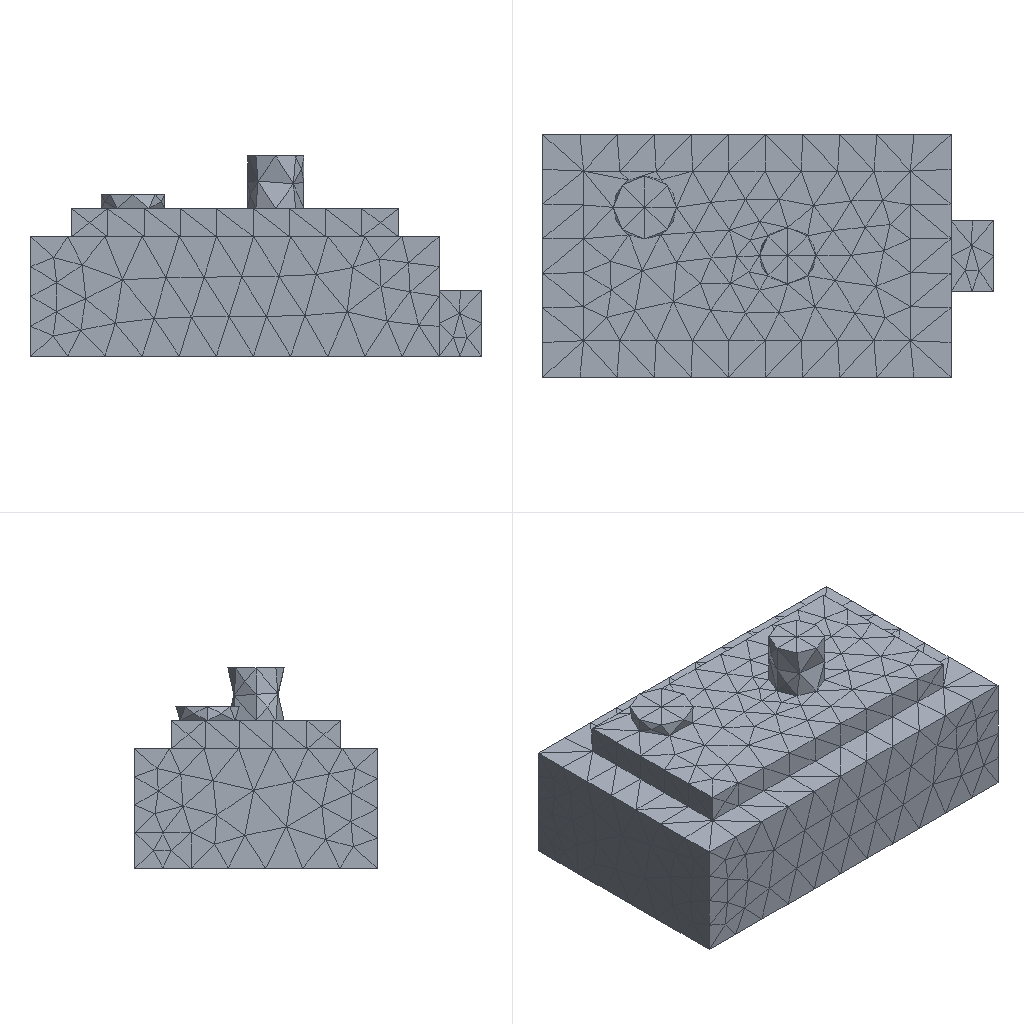Simulation study | ansys mapdl
Set-up summary:
category,name,step,type,value,unit,region
solver,ansys_mapdl
units,mm-N-s-tonne (MPa),,inferred,E=210000 density=
analysis,model,,static
mesh,nodes,,,4669
mesh,elements,,,2793
element_type,SOLID187,,,2793
material,mat 1,,E,210000
material,mat 1,,nu,0.3
load,,model,body load temp,,,all
load,,model,force,"1000 [dir=(0, 0, -1) n=93]",,node list
bc,,model,fixed,"[dofs=UX,UY,UZ n=4945]",,node list
Ansys APDL input file, long lists of numbers shortened:
/COM,ANSYS RELEASE 2026 R1           BUILD 26.1      UP20260202       09:08:28
/PREP7
/NOPR
/TITLE,2
ANTYPE, 0
*IF,_CDRDOFF,EQ,1,THEN     !if solid model was read in
_CDRDOFF=             !reset flag, numoffs already performed
*ELSE              !offset database for the following FE model
NUMOFF,NODE,     4669
NUMOFF,ELEM,     2793
NUMOFF,MAT ,        1
NUMOFF,TYPE,        1
*ENDIF
*SET,_RETURN ,  0.
*SET,_STATUS ,  0.
*SET,_UIQR   ,  93.
*SET,__FLOATPARAMETER__,  4669.
DOF,DELETE
ETBLOCK,        1,        1
(2i9,19a9)
        1      187        0        0        0        0        0        0        0        0        0        0        0        0        0        0        0        0        0        0        0
       -1
NBLOCK,6,SOLID,      4669,      4669
(3i9,6e21.13e3)
        1        0        0-4.2125000000000E+001 3.4500000000000E+001 1.0000000000000E+001
! (4668 more lines like these left out)
N,UNBL,LOC,       -1,
EBLOCK,19,SOLID,      2793,      2793
(19i10)
         1         1         1         1         0         0         0         0        10         0         1      1791      1792      1793      1794      2057      2058      2059      2060
! (5585 more lines like these left out)
        -1
MPTEMP,UNBL, 1, 1,  0.    ,
MPDATA,UNBL, 1,EX  ,       1, 1,  210000.000    ,
MPTEMP,UNBL, 1, 1,  0.    ,
MPDATA,UNBL, 1,NUXY,       1, 1, 0.3    ,
MPTEMP,UNBL, 1, 1,  0.    ,
MPDATA,UNBL, 1,PRXY,       1, 1, 0.3    ,
EXTOPT,ATTR,      0,      0,      0
EXTOPT,ESIZE,  0,  0.
EXTOPT,ACLEAR,      0
TREF,  0.
IRLF,  0
BFUNIF,TEMP,_TINY
ACEL,  0.    ,  0.    ,  0.
OMEGA,  0.    ,  0.    ,  0.
DOMEGA,  0.    ,  0.    ,  0.
CGLOC,  0.    ,  0.    ,  0.
CGOMEGA,  0.    ,  0.    ,  0.
DCGOMG,  0.    ,  0.    ,  0.
KUSE,     0
TIME,  0.
ALPHAD,  0.
BETAD,  0.
DMPRAT,  0.
DMPSTR,  0.
CRPLIM, 0.1    ,   0
CRPLIM,  0.    ,   1
NCNV,     0, 1.000000000E+12,     0,  0.    ,  0.
NEQIT,     0
ERESX,DEFA
DBLOCK,      4945
(i9,a6,2(pg16.9))
        1  UX    0.00000000      0.00000000
! (4944 more lines like these left out)
       -1
FBLOCK,        93
(i9,a6,2(pg16.9))
      922  FZ   -10.7526882      0.00000000
! (92 more lines like these left out)
       -1
/GO
FINISH
Results summary:
result,analysis_type_db,,,static,unstated
result,n_sets,,,1,unstated
result,load_steps[0].set,load_step=1,,1,unstated
result,load_steps[0].substep,load_step=1,,1,unstated
result,load_steps[0].time,load_step=1,,1,unstated
result,load_steps[0].freq,load_step=1,,1,unstated
result,load_steps[0].max_usum,load_step=1,,0.0005571,unstated
result,load_steps[0].max_seqv,load_step=1,,6.398,unstated
result,load_steps[0].reaction_sum.FX,load_step=1,,-1.03384e-12,unstated
result,load_steps[0].reaction_sum.FY,load_step=1,,-1.10929e-12,unstated
result,load_steps[0].reaction_sum.FZ,load_step=1,,1000,unstated
result,load_steps[0].reaction_sum.MX,load_step=1,,0,unstated
result,load_steps[0].reaction_sum.MY,load_step=1,,0,unstated
result,load_steps[0].reaction_sum.MZ,load_step=1,,0,unstated
result,convergence,,,results present for all listed sets,unstated